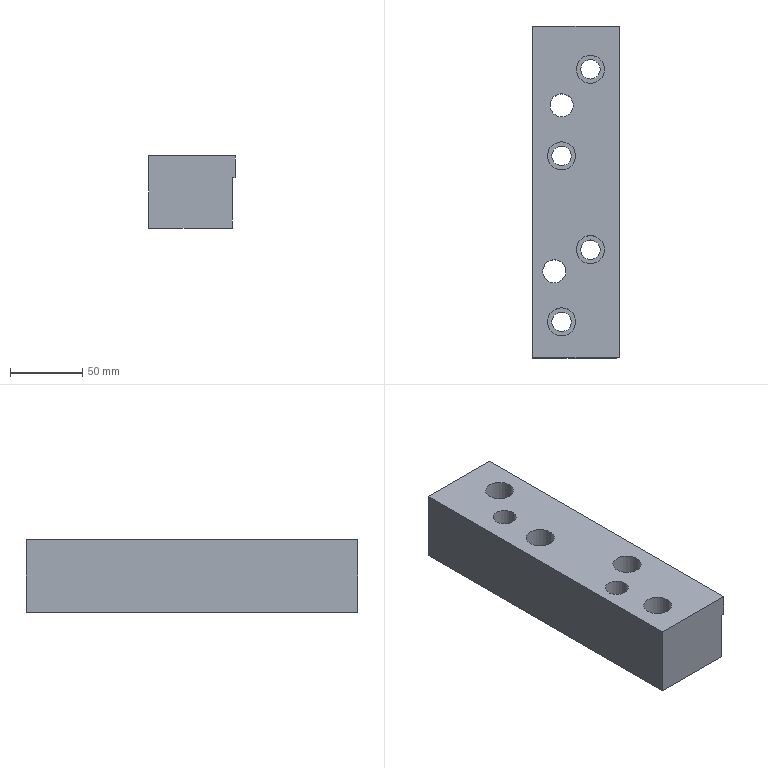Part | NX | features solid 2 | 1 solid | 22 faces | box 60 x 230 x 50 mm | volume 609615 mm3 | plane 12 | cylinder 10 | commonest cylinder face diameters 13.5 x4 19.5 x4 16 x2
STEP:
#1=CARTESIAN_POINT('',(1185.,-210.,-50.));
#2=VERTEX_POINT('',#1);
#3=CARTESIAN_POINT('',(1185.,-210.,0.));
#4=VERTEX_POINT('',#3);
#5=CARTESIAN_POINT('',(1185.,-210.,0.));
#6=DIRECTION('',(0.,0.,1.));
#7=VECTOR('',#6,1000.);
#8=LINE('',#5,#7);
#9=EDGE_CURVE('',#2,#4,#8,.T.);
#10=ORIENTED_EDGE('',*,*,#9,.F.);
#11=CARTESIAN_POINT('',(1185.,-440.,-50.));
#12=VERTEX_POINT('',#11);
#13=CARTESIAN_POINT('',(1185.,390.,-50.));
#14=DIRECTION('',(0.,1.,0.));
#15=VECTOR('',#14,1000.);
#16=LINE('',#13,#15);
#17=EDGE_CURVE('',#2,#12,#16,.F.);
#18=ORIENTED_EDGE('',*,*,#17,.T.);
#19=CARTESIAN_POINT('',(1185.,-440.,0.));
#20=VERTEX_POINT('',#19);
#21=CARTESIAN_POINT('',(1185.,-440.,0.));
#22=DIRECTION('',(0.,0.,1.));
#23=VECTOR('',#22,1000.);
#24=LINE('',#21,#23);
#25=EDGE_CURVE('',#20,#12,#24,.F.);
#26=ORIENTED_EDGE('',*,*,#25,.F.);
#27=CARTESIAN_POINT('',(1185.,390.,0.));
#28=DIRECTION('',(0.,1.,0.));
#29=VECTOR('',#28,1000.);
#30=LINE('',#27,#29);
#31=EDGE_CURVE('',#4,#20,#30,.F.);
#32=ORIENTED_EDGE('',*,*,#31,.F.);
#33=EDGE_LOOP('',(#10,#18,#26,#32));
#34=FACE_BOUND('',#33,.T.);
#35=CARTESIAN_POINT('',(1185.,390.,0.));
#36=DIRECTION('',(1.,0.,0.));
#37=DIRECTION('',(0.,0.,-1.));
#38=AXIS2_PLACEMENT_3D('',#35,#36,#37);
#39=PLANE('',#38);
#40=ADVANCED_FACE('',(#34),#39,.F.);
#41=CARTESIAN_POINT('',(1245.,-210.,-15.));
#42=VERTEX_POINT('',#41);
#43=CARTESIAN_POINT('',(1245.,-440.,-15.));
#44=VERTEX_POINT('',#43);
#45=CARTESIAN_POINT('',(1245.,250.,-15.));
#46=DIRECTION('',(0.,-1.,0.));
#47=VECTOR('',#46,1000.);
#48=LINE('',#45,#47);
#49=EDGE_CURVE('',#42,#44,#48,.T.);
#50=ORIENTED_EDGE('',*,*,#49,.F.);
#51=CARTESIAN_POINT('',(1245.,-210.,0.));
#52=VERTEX_POINT('',#51);
#53=CARTESIAN_POINT('',(1245.,-210.,0.));
#54=DIRECTION('',(0.,0.,1.));
#55=VECTOR('',#54,1000.);
#56=LINE('',#53,#55);
#57=EDGE_CURVE('',#42,#52,#56,.T.);
#58=ORIENTED_EDGE('',*,*,#57,.T.);
#59=CARTESIAN_POINT('',(1245.,-440.,0.));
#60=VERTEX_POINT('',#59);
#61=CARTESIAN_POINT('',(1245.,390.,0.));
#62=DIRECTION('',(0.,-1.,0.));
#63=VECTOR('',#62,1000.);
#64=LINE('',#61,#63);
#65=EDGE_CURVE('',#52,#60,#64,.T.);
#66=ORIENTED_EDGE('',*,*,#65,.T.);
#67=CARTESIAN_POINT('',(1245.,-440.,0.));
#68=DIRECTION('',(0.,0.,1.));
#69=VECTOR('',#68,1000.);
#70=LINE('',#67,#69);
#71=EDGE_CURVE('',#60,#44,#70,.F.);
#72=ORIENTED_EDGE('',*,*,#71,.T.);
#73=EDGE_LOOP('',(#50,#58,#66,#72));
#74=FACE_BOUND('',#73,.T.);
#75=CARTESIAN_POINT('',(1245.,390.,0.));
#76=DIRECTION('',(1.,0.,0.));
#77=DIRECTION('',(0.,0.,-1.));
#78=AXIS2_PLACEMENT_3D('',#75,#76,#77);
#79=PLANE('',#78);
#80=ADVANCED_FACE('',(#74),#79,.T.);
#81=CARTESIAN_POINT('',(1200.,-388.,-50.));
#82=VERTEX_POINT('',#81);
#83=CARTESIAN_POINT('',(1200.,-380.,-50.));
#84=DIRECTION('',(0.,0.,1.));
#85=DIRECTION('',(0.,-1.,0.));
#86=AXIS2_PLACEMENT_3D('',#83,#84,#85);
#87=CIRCLE('',#86,8.);
#88=EDGE_CURVE('',#82,#82,#87,.T.);
#89=ORIENTED_EDGE('',*,*,#88,.T.);
#90=EDGE_LOOP('',(#89));
#91=FACE_BOUND('',#90,.T.);
#92=CARTESIAN_POINT('',(1205.,-273.,-50.));
#93=VERTEX_POINT('',#92);
#94=CARTESIAN_POINT('',(1205.,-265.,-50.));
#95=DIRECTION('',(0.,0.,1.));
#96=DIRECTION('',(0.,-1.,0.));
#97=AXIS2_PLACEMENT_3D('',#94,#95,#96);
#98=CIRCLE('',#97,8.);
#99=EDGE_CURVE('',#93,#93,#98,.T.);
#100=ORIENTED_EDGE('',*,*,#99,.T.);
#101=EDGE_LOOP('',(#100));
#102=FACE_BOUND('',#101,.T.);
#103=CARTESIAN_POINT('',(1205.,-421.75,-50.));
#104=VERTEX_POINT('',#103);
#105=CARTESIAN_POINT('',(1205.,-415.,-50.));
#106=DIRECTION('',(0.,0.,1.));
#107=DIRECTION('',(0.,-1.,0.));
#108=AXIS2_PLACEMENT_3D('',#105,#106,#107);
#109=CIRCLE('',#108,6.75);
#110=EDGE_CURVE('',#104,#104,#109,.T.);
#111=ORIENTED_EDGE('',*,*,#110,.T.);
#112=EDGE_LOOP('',(#111));
#113=FACE_BOUND('',#112,.T.);
#114=CARTESIAN_POINT('',(1225.,-371.75,-50.));
#115=VERTEX_POINT('',#114);
#116=CARTESIAN_POINT('',(1225.,-365.,-50.));
#117=DIRECTION('',(0.,0.,1.));
#118=DIRECTION('',(0.,-1.,0.));
#119=AXIS2_PLACEMENT_3D('',#116,#117,#118);
#120=CIRCLE('',#119,6.75);
#121=EDGE_CURVE('',#115,#115,#120,.T.);
#122=ORIENTED_EDGE('',*,*,#121,.T.);
#123=EDGE_LOOP('',(#122));
#124=FACE_BOUND('',#123,.T.);
#125=CARTESIAN_POINT('',(1205.,-306.75,-50.));
#126=VERTEX_POINT('',#125);
#127=CARTESIAN_POINT('',(1205.,-300.,-50.));
#128=DIRECTION('',(0.,0.,1.));
#129=DIRECTION('',(0.,-1.,0.));
#130=AXIS2_PLACEMENT_3D('',#127,#128,#129);
#131=CIRCLE('',#130,6.75);
#132=EDGE_CURVE('',#126,#126,#131,.T.);
#133=ORIENTED_EDGE('',*,*,#132,.T.);
#134=EDGE_LOOP('',(#133));
#135=FACE_BOUND('',#134,.T.);
#136=CARTESIAN_POINT('',(1225.,-246.75,-50.));
#137=VERTEX_POINT('',#136);
#138=CARTESIAN_POINT('',(1225.,-240.,-50.));
#139=DIRECTION('',(0.,0.,1.));
#140=DIRECTION('',(0.,-1.,0.));
#141=AXIS2_PLACEMENT_3D('',#138,#139,#140);
#142=CIRCLE('',#141,6.75);
#143=EDGE_CURVE('',#137,#137,#142,.T.);
#144=ORIENTED_EDGE('',*,*,#143,.T.);
#145=EDGE_LOOP('',(#144));
#146=FACE_BOUND('',#145,.T.);
#147=CARTESIAN_POINT('',(1243.,-210.,-50.));
#148=VERTEX_POINT('',#147);
#149=CARTESIAN_POINT('',(1245.,-210.,-50.));
#150=DIRECTION('',(-1.,0.,0.));
#151=VECTOR('',#150,1000.);
#152=LINE('',#149,#151);
#153=EDGE_CURVE('',#148,#2,#152,.T.);
#154=ORIENTED_EDGE('',*,*,#153,.F.);
#155=CARTESIAN_POINT('',(1243.,-440.,-50.));
#156=VERTEX_POINT('',#155);
#157=CARTESIAN_POINT('',(1243.,390.,-50.));
#158=DIRECTION('',(0.,-1.,0.));
#159=VECTOR('',#158,1000.);
#160=LINE('',#157,#159);
#161=EDGE_CURVE('',#148,#156,#160,.T.);
#162=ORIENTED_EDGE('',*,*,#161,.T.);
#163=CARTESIAN_POINT('',(1245.,-440.,-50.));
#164=DIRECTION('',(1.,0.,0.));
#165=VECTOR('',#164,1000.);
#166=LINE('',#163,#165);
#167=EDGE_CURVE('',#156,#12,#166,.F.);
#168=ORIENTED_EDGE('',*,*,#167,.T.);
#169=ORIENTED_EDGE('',*,*,#17,.F.);
#170=EDGE_LOOP('',(#154,#162,#168,#169));
#171=FACE_BOUND('',#170,.T.);
#172=CARTESIAN_POINT('',(1245.,390.,-50.));
#173=DIRECTION('',(0.,0.,1.));
#174=DIRECTION('',(0.,-1.,0.));
#175=AXIS2_PLACEMENT_3D('',#172,#173,#174);
#176=PLANE('',#175);
#177=ADVANCED_FACE('',(#91,#102,#113,#124,#135,#146,#171),#176,.F.);
#178=CARTESIAN_POINT('',(1200.,-388.,0.));
#179=VERTEX_POINT('',#178);
#180=CARTESIAN_POINT('',(1200.,-380.,0.));
#181=DIRECTION('',(0.,0.,1.));
#182=DIRECTION('',(0.,-1.,0.));
#183=AXIS2_PLACEMENT_3D('',#180,#181,#182);
#184=CIRCLE('',#183,8.);
#185=EDGE_CURVE('',#179,#179,#184,.F.);
#186=ORIENTED_EDGE('',*,*,#185,.T.);
#187=EDGE_LOOP('',(#186));
#188=FACE_BOUND('',#187,.T.);
#189=CARTESIAN_POINT('',(1205.,-273.,0.));
#190=VERTEX_POINT('',#189);
#191=CARTESIAN_POINT('',(1205.,-265.,0.));
#192=DIRECTION('',(0.,0.,1.));
#193=DIRECTION('',(0.,-1.,0.));
#194=AXIS2_PLACEMENT_3D('',#191,#192,#193);
#195=CIRCLE('',#194,8.);
#196=EDGE_CURVE('',#190,#190,#195,.F.);
#197=ORIENTED_EDGE('',*,*,#196,.T.);
#198=EDGE_LOOP('',(#197));
#199=FACE_BOUND('',#198,.T.);
#200=CARTESIAN_POINT('',(1225.,-249.75,0.));
#201=VERTEX_POINT('',#200);
#202=CARTESIAN_POINT('',(1225.,-240.,0.));
#203=DIRECTION('',(0.,0.,1.));
#204=DIRECTION('',(0.,-1.,0.));
#205=AXIS2_PLACEMENT_3D('',#202,#203,#204);
#206=CIRCLE('',#205,9.75);
#207=EDGE_CURVE('',#201,#201,#206,.F.);
#208=ORIENTED_EDGE('',*,*,#207,.T.);
#209=EDGE_LOOP('',(#208));
#210=FACE_BOUND('',#209,.T.);
#211=CARTESIAN_POINT('',(1205.,-309.75,0.));
#212=VERTEX_POINT('',#211);
#213=CARTESIAN_POINT('',(1205.,-300.,0.));
#214=DIRECTION('',(0.,0.,1.));
#215=DIRECTION('',(0.,-1.,0.));
#216=AXIS2_PLACEMENT_3D('',#213,#214,#215);
#217=CIRCLE('',#216,9.75);
#218=EDGE_CURVE('',#212,#212,#217,.F.);
#219=ORIENTED_EDGE('',*,*,#218,.T.);
#220=EDGE_LOOP('',(#219));
#221=FACE_BOUND('',#220,.T.);
#222=CARTESIAN_POINT('',(1225.,-374.75,0.));
#223=VERTEX_POINT('',#222);
#224=CARTESIAN_POINT('',(1225.,-365.,0.));
#225=DIRECTION('',(0.,0.,1.));
#226=DIRECTION('',(0.,-1.,0.));
#227=AXIS2_PLACEMENT_3D('',#224,#225,#226);
#228=CIRCLE('',#227,9.75);
#229=EDGE_CURVE('',#223,#223,#228,.F.);
#230=ORIENTED_EDGE('',*,*,#229,.T.);
#231=EDGE_LOOP('',(#230));
#232=FACE_BOUND('',#231,.T.);
#233=CARTESIAN_POINT('',(1205.,-424.75,0.));
#234=VERTEX_POINT('',#233);
#235=CARTESIAN_POINT('',(1205.,-415.,0.));
#236=DIRECTION('',(0.,0.,1.));
#237=DIRECTION('',(0.,-1.,0.));
#238=AXIS2_PLACEMENT_3D('',#235,#236,#237);
#239=CIRCLE('',#238,9.75);
#240=EDGE_CURVE('',#234,#234,#239,.F.);
#241=ORIENTED_EDGE('',*,*,#240,.T.);
#242=EDGE_LOOP('',(#241));
#243=FACE_BOUND('',#242,.T.);
#244=CARTESIAN_POINT('',(1245.,-210.,0.));
#245=DIRECTION('',(-1.,0.,0.));
#246=VECTOR('',#245,1000.);
#247=LINE('',#244,#246);
#248=EDGE_CURVE('',#4,#52,#247,.F.);
#249=ORIENTED_EDGE('',*,*,#248,.F.);
#250=ORIENTED_EDGE('',*,*,#31,.T.);
#251=CARTESIAN_POINT('',(1245.,-440.,0.));
#252=DIRECTION('',(-1.,0.,0.));
#253=VECTOR('',#252,1000.);
#254=LINE('',#251,#253);
#255=EDGE_CURVE('',#60,#20,#254,.T.);
#256=ORIENTED_EDGE('',*,*,#255,.F.);
#257=ORIENTED_EDGE('',*,*,#65,.F.);
#258=EDGE_LOOP('',(#249,#250,#256,#257));
#259=FACE_BOUND('',#258,.T.);
#260=CARTESIAN_POINT('',(1245.,390.,0.));
#261=DIRECTION('',(0.,0.,1.));
#262=DIRECTION('',(0.,-1.,0.));
#263=AXIS2_PLACEMENT_3D('',#260,#261,#262);
#264=PLANE('',#263);
#265=ADVANCED_FACE('',(#188,#199,#210,#221,#232,#243,#259),#264,.T.);
#266=CARTESIAN_POINT('',(1243.,-210.,-15.));
#267=VERTEX_POINT('',#266);
#268=CARTESIAN_POINT('',(1243.,-210.,-100.));
#269=DIRECTION('',(0.,0.,-1.));
#270=VECTOR('',#269,1000.);
#271=LINE('',#268,#270);
#272=EDGE_CURVE('',#267,#148,#271,.T.);
#273=ORIENTED_EDGE('',*,*,#272,.F.);
#274=CARTESIAN_POINT('',(1243.,-440.,-15.));
#275=VERTEX_POINT('',#274);
#276=CARTESIAN_POINT('',(1243.,250.,-15.));
#277=DIRECTION('',(0.,1.,0.));
#278=VECTOR('',#277,1000.);
#279=LINE('',#276,#278);
#280=EDGE_CURVE('',#267,#275,#279,.F.);
#281=ORIENTED_EDGE('',*,*,#280,.T.);
#282=CARTESIAN_POINT('',(1243.,-440.,0.));
#283=DIRECTION('',(0.,0.,-1.));
#284=VECTOR('',#283,1000.);
#285=LINE('',#282,#284);
#286=EDGE_CURVE('',#156,#275,#285,.F.);
#287=ORIENTED_EDGE('',*,*,#286,.F.);
#288=ORIENTED_EDGE('',*,*,#161,.F.);
#289=EDGE_LOOP('',(#273,#281,#287,#288));
#290=FACE_BOUND('',#289,.T.);
#291=CARTESIAN_POINT('',(1243.,250.,-100.));
#292=DIRECTION('',(-1.,0.,0.));
#293=DIRECTION('',(0.,0.,1.));
#294=AXIS2_PLACEMENT_3D('',#291,#292,#293);
#295=PLANE('',#294);
#296=ADVANCED_FACE('',(#290),#295,.F.);
#297=CARTESIAN_POINT('',(1245.,-210.,-15.));
#298=DIRECTION('',(1.,0.,0.));
#299=VECTOR('',#298,1000.);
#300=LINE('',#297,#299);
#301=EDGE_CURVE('',#42,#267,#300,.F.);
#302=ORIENTED_EDGE('',*,*,#301,.F.);
#303=ORIENTED_EDGE('',*,*,#49,.T.);
#304=CARTESIAN_POINT('',(1245.,-440.,-15.));
#305=DIRECTION('',(-1.,0.,0.));
#306=VECTOR('',#305,1000.);
#307=LINE('',#304,#306);
#308=EDGE_CURVE('',#44,#275,#307,.T.);
#309=ORIENTED_EDGE('',*,*,#308,.T.);
#310=ORIENTED_EDGE('',*,*,#280,.F.);
#311=EDGE_LOOP('',(#302,#303,#309,#310));
#312=FACE_BOUND('',#311,.T.);
#313=CARTESIAN_POINT('',(1245.,250.,-15.));
#314=DIRECTION('',(0.,0.,-1.));
#315=DIRECTION('',(0.,-1.,0.));
#316=AXIS2_PLACEMENT_3D('',#313,#314,#315);
#317=PLANE('',#316);
#318=ADVANCED_FACE('',(#312),#317,.T.);
#319=ORIENTED_EDGE('',*,*,#286,.T.);
#320=ORIENTED_EDGE('',*,*,#308,.F.);
#321=ORIENTED_EDGE('',*,*,#71,.F.);
#322=ORIENTED_EDGE('',*,*,#255,.T.);
#323=ORIENTED_EDGE('',*,*,#25,.T.);
#324=ORIENTED_EDGE('',*,*,#167,.F.);
#325=EDGE_LOOP('',(#319,#320,#321,#322,#323,#324));
#326=FACE_BOUND('',#325,.T.);
#327=CARTESIAN_POINT('',(1245.,-440.,0.));
#328=DIRECTION('',(0.,-1.,0.));
#329=DIRECTION('',(0.,0.,-1.));
#330=AXIS2_PLACEMENT_3D('',#327,#328,#329);
#331=PLANE('',#330);
#332=ADVANCED_FACE('',(#326),#331,.T.);
#333=ORIENTED_EDGE('',*,*,#9,.T.);
#334=ORIENTED_EDGE('',*,*,#248,.T.);
#335=ORIENTED_EDGE('',*,*,#57,.F.);
#336=ORIENTED_EDGE('',*,*,#301,.T.);
#337=ORIENTED_EDGE('',*,*,#272,.T.);
#338=ORIENTED_EDGE('',*,*,#153,.T.);
#339=EDGE_LOOP('',(#333,#334,#335,#336,#337,#338));
#340=FACE_BOUND('',#339,.T.);
#341=CARTESIAN_POINT('',(1185.,-210.,0.));
#342=DIRECTION('',(0.,1.,0.));
#343=DIRECTION('',(0.,0.,1.));
#344=AXIS2_PLACEMENT_3D('',#341,#342,#343);
#345=PLANE('',#344);
#346=ADVANCED_FACE('',(#340),#345,.T.);
#347=CARTESIAN_POINT('',(1225.,-233.25,-25.));
#348=VERTEX_POINT('',#347);
#349=CARTESIAN_POINT('',(1225.,-240.,-25.));
#350=DIRECTION('',(0.,0.,-1.));
#351=DIRECTION('',(0.,1.,0.));
#352=AXIS2_PLACEMENT_3D('',#349,#350,#351);
#353=CIRCLE('',#352,6.75);
#354=EDGE_CURVE('',#348,#348,#353,.F.);
#355=ORIENTED_EDGE('',*,*,#354,.T.);
#356=EDGE_LOOP('',(#355));
#357=FACE_BOUND('',#356,.T.);
#358=ORIENTED_EDGE('',*,*,#143,.F.);
#359=EDGE_LOOP('',(#358));
#360=FACE_BOUND('',#359,.T.);
#361=CARTESIAN_POINT('',(1225.,-240.,75.));
#362=DIRECTION('',(0.,0.,-1.));
#363=DIRECTION('',(-1.,0.,0.));
#364=AXIS2_PLACEMENT_3D('',#361,#362,#363);
#365=CYLINDRICAL_SURFACE('',#364,6.75);
#366=ADVANCED_FACE('',(#357,#360),#365,.F.);
#367=CARTESIAN_POINT('',(1205.,-293.25,-25.));
#368=VERTEX_POINT('',#367);
#369=CARTESIAN_POINT('',(1205.,-300.,-25.));
#370=DIRECTION('',(0.,0.,-1.));
#371=DIRECTION('',(0.,1.,0.));
#372=AXIS2_PLACEMENT_3D('',#369,#370,#371);
#373=CIRCLE('',#372,6.75);
#374=EDGE_CURVE('',#368,#368,#373,.F.);
#375=ORIENTED_EDGE('',*,*,#374,.T.);
#376=EDGE_LOOP('',(#375));
#377=FACE_BOUND('',#376,.T.);
#378=ORIENTED_EDGE('',*,*,#132,.F.);
#379=EDGE_LOOP('',(#378));
#380=FACE_BOUND('',#379,.T.);
#381=CARTESIAN_POINT('',(1205.,-300.,75.));
#382=DIRECTION('',(0.,0.,-1.));
#383=DIRECTION('',(-1.,0.,0.));
#384=AXIS2_PLACEMENT_3D('',#381,#382,#383);
#385=CYLINDRICAL_SURFACE('',#384,6.75);
#386=ADVANCED_FACE('',(#377,#380),#385,.F.);
#387=CARTESIAN_POINT('',(1225.,-358.25,-25.));
#388=VERTEX_POINT('',#387);
#389=CARTESIAN_POINT('',(1225.,-365.,-25.));
#390=DIRECTION('',(0.,0.,-1.));
#391=DIRECTION('',(0.,1.,0.));
#392=AXIS2_PLACEMENT_3D('',#389,#390,#391);
#393=CIRCLE('',#392,6.75);
#394=EDGE_CURVE('',#388,#388,#393,.F.);
#395=ORIENTED_EDGE('',*,*,#394,.T.);
#396=EDGE_LOOP('',(#395));
#397=FACE_BOUND('',#396,.T.);
#398=ORIENTED_EDGE('',*,*,#121,.F.);
#399=EDGE_LOOP('',(#398));
#400=FACE_BOUND('',#399,.T.);
#401=CARTESIAN_POINT('',(1225.,-365.,75.));
#402=DIRECTION('',(0.,0.,-1.));
#403=DIRECTION('',(-1.,0.,0.));
#404=AXIS2_PLACEMENT_3D('',#401,#402,#403);
#405=CYLINDRICAL_SURFACE('',#404,6.75);
#406=ADVANCED_FACE('',(#397,#400),#405,.F.);
#407=CARTESIAN_POINT('',(1205.,-408.25,-25.));
#408=VERTEX_POINT('',#407);
#409=CARTESIAN_POINT('',(1205.,-415.,-25.));
#410=DIRECTION('',(0.,0.,-1.));
#411=DIRECTION('',(0.,1.,0.));
#412=AXIS2_PLACEMENT_3D('',#409,#410,#411);
#413=CIRCLE('',#412,6.75);
#414=EDGE_CURVE('',#408,#408,#413,.F.);
#415=ORIENTED_EDGE('',*,*,#414,.T.);
#416=EDGE_LOOP('',(#415));
#417=FACE_BOUND('',#416,.T.);
#418=ORIENTED_EDGE('',*,*,#110,.F.);
#419=EDGE_LOOP('',(#418));
#420=FACE_BOUND('',#419,.T.);
#421=CARTESIAN_POINT('',(1205.,-415.,75.));
#422=DIRECTION('',(0.,0.,-1.));
#423=DIRECTION('',(-1.,0.,0.));
#424=AXIS2_PLACEMENT_3D('',#421,#422,#423);
#425=CYLINDRICAL_SURFACE('',#424,6.75);
#426=ADVANCED_FACE('',(#417,#420),#425,.F.);
#427=CARTESIAN_POINT('',(1205.,-405.25,-25.));
#428=VERTEX_POINT('',#427);
#429=CARTESIAN_POINT('',(1205.,-415.,-25.));
#430=DIRECTION('',(0.,0.,-1.));
#431=DIRECTION('',(0.,1.,0.));
#432=AXIS2_PLACEMENT_3D('',#429,#430,#431);
#433=CIRCLE('',#432,9.75);
#434=EDGE_CURVE('',#428,#428,#433,.T.);
#435=ORIENTED_EDGE('',*,*,#434,.T.);
#436=EDGE_LOOP('',(#435));
#437=FACE_BOUND('',#436,.T.);
#438=ORIENTED_EDGE('',*,*,#240,.F.);
#439=EDGE_LOOP('',(#438));
#440=FACE_BOUND('',#439,.T.);
#441=CARTESIAN_POINT('',(1205.,-415.,75.));
#442=DIRECTION('',(0.,0.,-1.));
#443=DIRECTION('',(-1.,0.,0.));
#444=AXIS2_PLACEMENT_3D('',#441,#442,#443);
#445=CYLINDRICAL_SURFACE('',#444,9.75);
#446=ADVANCED_FACE('',(#437,#440),#445,.F.);
#447=ORIENTED_EDGE('',*,*,#434,.F.);
#448=EDGE_LOOP('',(#447));
#449=FACE_BOUND('',#448,.T.);
#450=ORIENTED_EDGE('',*,*,#414,.F.);
#451=EDGE_LOOP('',(#450));
#452=FACE_BOUND('',#451,.T.);
#453=CARTESIAN_POINT('',(1205.,-415.,-25.));
#454=DIRECTION('',(0.,0.,-1.));
#455=DIRECTION('',(0.,1.,0.));
#456=AXIS2_PLACEMENT_3D('',#453,#454,#455);
#457=PLANE('',#456);
#458=ADVANCED_FACE('',(#449,#452),#457,.F.);
#459=CARTESIAN_POINT('',(1225.,-355.25,-25.));
#460=VERTEX_POINT('',#459);
#461=CARTESIAN_POINT('',(1225.,-365.,-25.));
#462=DIRECTION('',(0.,0.,-1.));
#463=DIRECTION('',(0.,1.,0.));
#464=AXIS2_PLACEMENT_3D('',#461,#462,#463);
#465=CIRCLE('',#464,9.75);
#466=EDGE_CURVE('',#460,#460,#465,.T.);
#467=ORIENTED_EDGE('',*,*,#466,.T.);
#468=EDGE_LOOP('',(#467));
#469=FACE_BOUND('',#468,.T.);
#470=ORIENTED_EDGE('',*,*,#229,.F.);
#471=EDGE_LOOP('',(#470));
#472=FACE_BOUND('',#471,.T.);
#473=CARTESIAN_POINT('',(1225.,-365.,75.));
#474=DIRECTION('',(0.,0.,-1.));
#475=DIRECTION('',(-1.,0.,0.));
#476=AXIS2_PLACEMENT_3D('',#473,#474,#475);
#477=CYLINDRICAL_SURFACE('',#476,9.75);
#478=ADVANCED_FACE('',(#469,#472),#477,.F.);
#479=ORIENTED_EDGE('',*,*,#466,.F.);
#480=EDGE_LOOP('',(#479));
#481=FACE_BOUND('',#480,.T.);
#482=ORIENTED_EDGE('',*,*,#394,.F.);
#483=EDGE_LOOP('',(#482));
#484=FACE_BOUND('',#483,.T.);
#485=CARTESIAN_POINT('',(1225.,-365.,-25.));
#486=DIRECTION('',(0.,0.,-1.));
#487=DIRECTION('',(0.,1.,0.));
#488=AXIS2_PLACEMENT_3D('',#485,#486,#487);
#489=PLANE('',#488);
#490=ADVANCED_FACE('',(#481,#484),#489,.F.);
#491=CARTESIAN_POINT('',(1205.,-290.25,-25.));
#492=VERTEX_POINT('',#491);
#493=CARTESIAN_POINT('',(1205.,-300.,-25.));
#494=DIRECTION('',(0.,0.,-1.));
#495=DIRECTION('',(0.,1.,0.));
#496=AXIS2_PLACEMENT_3D('',#493,#494,#495);
#497=CIRCLE('',#496,9.75);
#498=EDGE_CURVE('',#492,#492,#497,.T.);
#499=ORIENTED_EDGE('',*,*,#498,.T.);
#500=EDGE_LOOP('',(#499));
#501=FACE_BOUND('',#500,.T.);
#502=ORIENTED_EDGE('',*,*,#218,.F.);
#503=EDGE_LOOP('',(#502));
#504=FACE_BOUND('',#503,.T.);
#505=CARTESIAN_POINT('',(1205.,-300.,75.));
#506=DIRECTION('',(0.,0.,-1.));
#507=DIRECTION('',(-1.,0.,0.));
#508=AXIS2_PLACEMENT_3D('',#505,#506,#507);
#509=CYLINDRICAL_SURFACE('',#508,9.75);
#510=ADVANCED_FACE('',(#501,#504),#509,.F.);
#511=ORIENTED_EDGE('',*,*,#498,.F.);
#512=EDGE_LOOP('',(#511));
#513=FACE_BOUND('',#512,.T.);
#514=ORIENTED_EDGE('',*,*,#374,.F.);
#515=EDGE_LOOP('',(#514));
#516=FACE_BOUND('',#515,.T.);
#517=CARTESIAN_POINT('',(1205.,-300.,-25.));
#518=DIRECTION('',(0.,0.,-1.));
#519=DIRECTION('',(0.,1.,0.));
#520=AXIS2_PLACEMENT_3D('',#517,#518,#519);
#521=PLANE('',#520);
#522=ADVANCED_FACE('',(#513,#516),#521,.F.);
#523=CARTESIAN_POINT('',(1225.,-230.25,-25.));
#524=VERTEX_POINT('',#523);
#525=CARTESIAN_POINT('',(1225.,-240.,-25.));
#526=DIRECTION('',(0.,0.,-1.));
#527=DIRECTION('',(0.,1.,0.));
#528=AXIS2_PLACEMENT_3D('',#525,#526,#527);
#529=CIRCLE('',#528,9.75);
#530=EDGE_CURVE('',#524,#524,#529,.T.);
#531=ORIENTED_EDGE('',*,*,#530,.T.);
#532=EDGE_LOOP('',(#531));
#533=FACE_BOUND('',#532,.T.);
#534=ORIENTED_EDGE('',*,*,#207,.F.);
#535=EDGE_LOOP('',(#534));
#536=FACE_BOUND('',#535,.T.);
#537=CARTESIAN_POINT('',(1225.,-240.,75.));
#538=DIRECTION('',(0.,0.,-1.));
#539=DIRECTION('',(-1.,0.,0.));
#540=AXIS2_PLACEMENT_3D('',#537,#538,#539);
#541=CYLINDRICAL_SURFACE('',#540,9.75);
#542=ADVANCED_FACE('',(#533,#536),#541,.F.);
#543=ORIENTED_EDGE('',*,*,#530,.F.);
#544=EDGE_LOOP('',(#543));
#545=FACE_BOUND('',#544,.T.);
#546=ORIENTED_EDGE('',*,*,#354,.F.);
#547=EDGE_LOOP('',(#546));
#548=FACE_BOUND('',#547,.T.);
#549=CARTESIAN_POINT('',(1225.,-240.,-25.));
#550=DIRECTION('',(0.,0.,-1.));
#551=DIRECTION('',(0.,1.,0.));
#552=AXIS2_PLACEMENT_3D('',#549,#550,#551);
#553=PLANE('',#552);
#554=ADVANCED_FACE('',(#545,#548),#553,.F.);
#555=ORIENTED_EDGE('',*,*,#196,.F.);
#556=EDGE_LOOP('',(#555));
#557=FACE_BOUND('',#556,.T.);
#558=ORIENTED_EDGE('',*,*,#99,.F.);
#559=EDGE_LOOP('',(#558));
#560=FACE_BOUND('',#559,.T.);
#561=CARTESIAN_POINT('',(1205.,-265.,100.));
#562=DIRECTION('',(0.,0.,-1.));
#563=DIRECTION('',(-1.,0.,0.));
#564=AXIS2_PLACEMENT_3D('',#561,#562,#563);
#565=CYLINDRICAL_SURFACE('',#564,8.);
#566=ADVANCED_FACE('',(#557,#560),#565,.F.);
#567=ORIENTED_EDGE('',*,*,#185,.F.);
#568=EDGE_LOOP('',(#567));
#569=FACE_BOUND('',#568,.T.);
#570=ORIENTED_EDGE('',*,*,#88,.F.);
#571=EDGE_LOOP('',(#570));
#572=FACE_BOUND('',#571,.T.);
#573=CARTESIAN_POINT('',(1200.,-380.,100.));
#574=DIRECTION('',(0.,0.,-1.));
#575=DIRECTION('',(-1.,0.,0.));
#576=AXIS2_PLACEMENT_3D('',#573,#574,#575);
#577=CYLINDRICAL_SURFACE('',#576,8.);
#578=ADVANCED_FACE('',(#569,#572),#577,.F.);
#579=CLOSED_SHELL('',(#40,#80,#177,#265,#296,#318,#332,#346,#366,#386,#406,#426,#446,#458,#478,#490,#510,#522,#542,#554,#566,#578));
#580=MANIFOLD_SOLID_BREP('',#579);
#581=(LENGTH_UNIT()NAMED_UNIT(*)SI_UNIT(.MILLI.,.METRE.));
#582=UNCERTAINTY_MEASURE_WITH_UNIT(LENGTH_MEASURE(0.00001),#581,'','');
#583=(NAMED_UNIT(*)PLANE_ANGLE_UNIT()SI_UNIT($,.RADIAN.));
#584=(NAMED_UNIT(*)SI_UNIT($,.STERADIAN.)SOLID_ANGLE_UNIT());
#585=(GEOMETRIC_REPRESENTATION_CONTEXT(3)GLOBAL_UNCERTAINTY_ASSIGNED_CONTEXT((#582))GLOBAL_UNIT_ASSIGNED_CONTEXT((#581,#583,#584))REPRESENTATION_CONTEXT('',''));
#586=ADVANCED_BREP_SHAPE_REPRESENTATION('',(#580),#585);